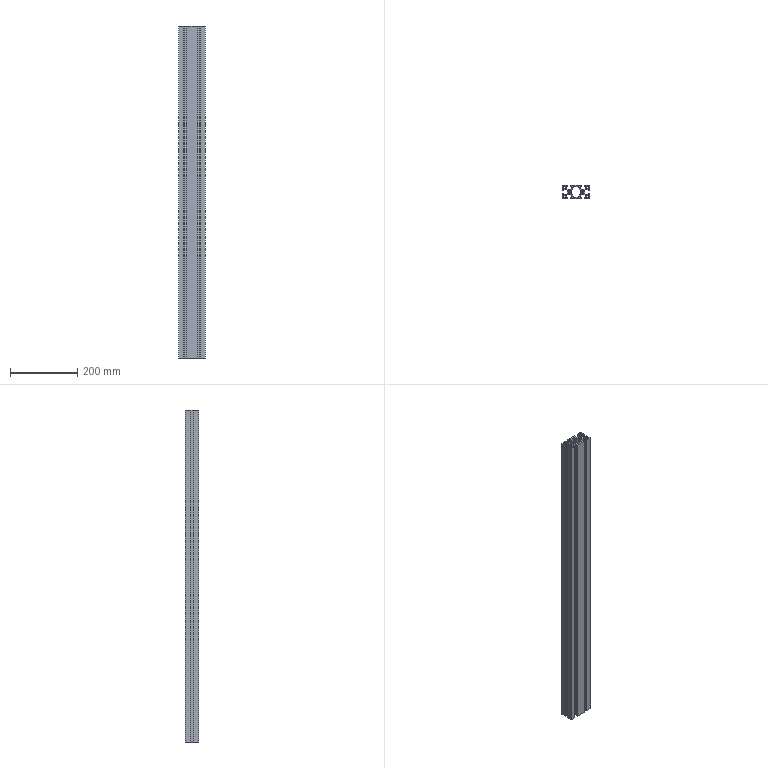Part | NX | 1 solid | 88 faces | box 80 x 40 x 991 mm | volume 1200573 mm3 | plane 78 | cylinder 10 | commonest cylinder face diameters 6 x4 8 x4 6.75 x2